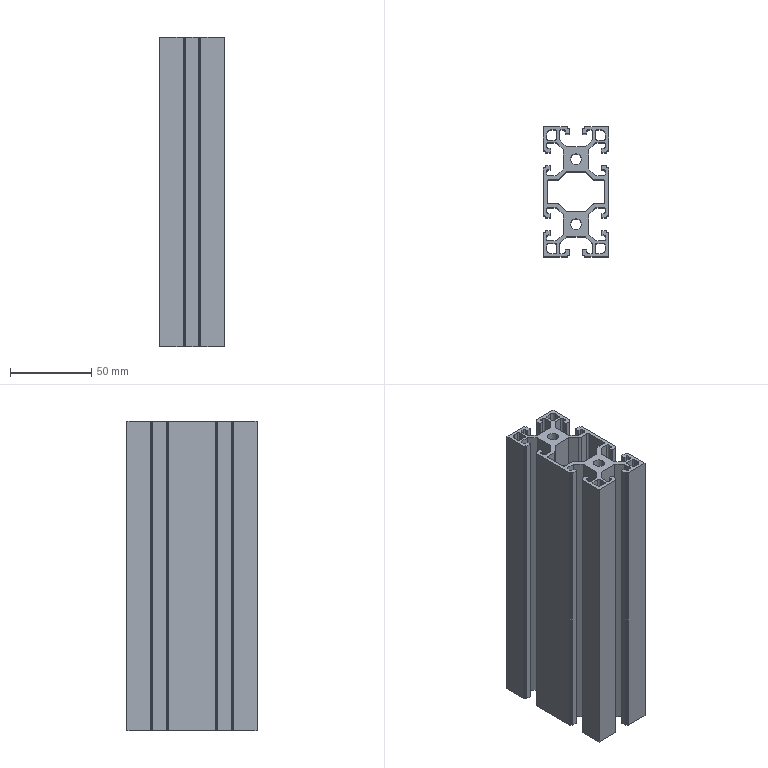Part | SolidWorks | features 3DProfileFeature 1, Extrusion 1, HoleWzd 1 | 1 solid | 276 faces | box 40 x 80 x 190 mm | volume 210236 mm3 | plane 142 | cylinder 134 | commonest cylinder face diameters 0.6 x70 2 x40 0.4 x12 4 x4 5 x4 6.8 x4